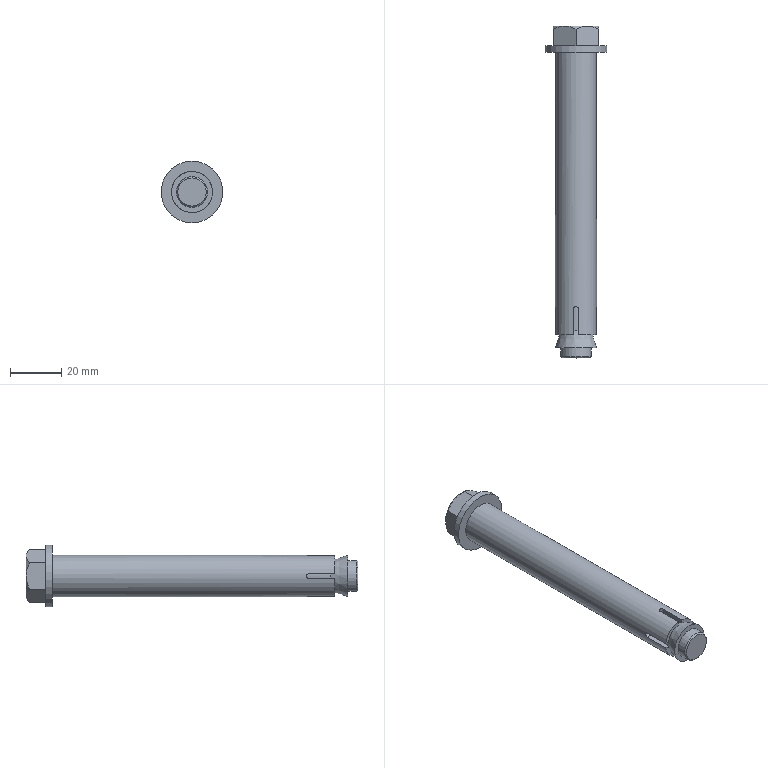Part | STEP file | Cone-head expansion bolt (ZM type) M12×110 A2-70 GBT22795 (ZM) - 2008_Default<As Machined> | 1 solid | 43 faces | box 24 x 129.18 x 24 mm | volume 26435 mm3 | plane 23 | cylinder 11 | cone 9 | commonest cylinder face diameters 12 x5 2 x4 16 x1 24 x1